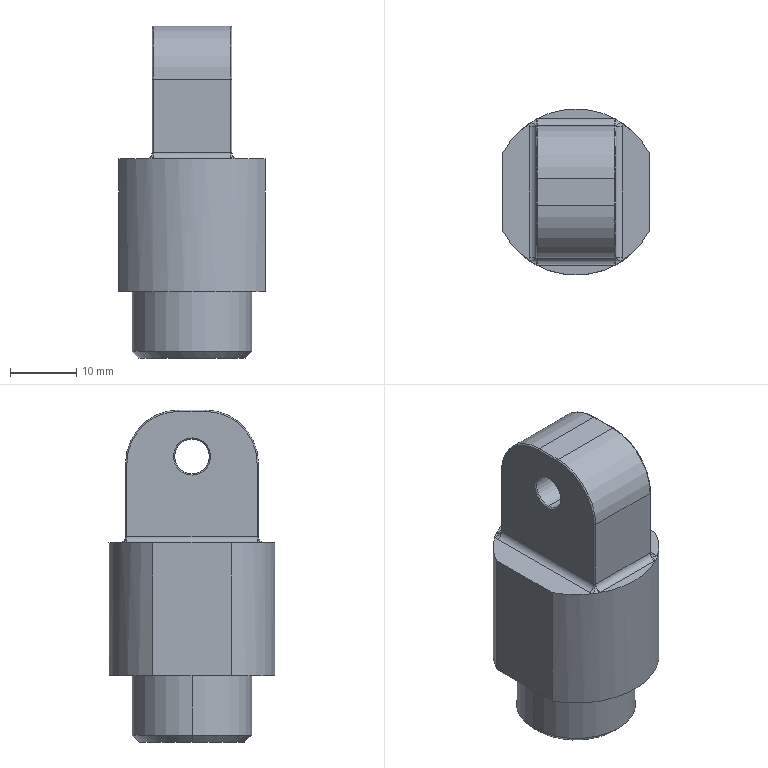Part | NX | features BREP 1 | 1 solid | 53 faces | box 22 x 25 x 50 mm | volume 16082 mm3 | cylinder 18 | plane 13 | torus 12 | cone 6 | spline 4 | commonest cylinder face diameters 0.4 x6 2 x4 5.2 x2 16 x2 18 x2 25 x2